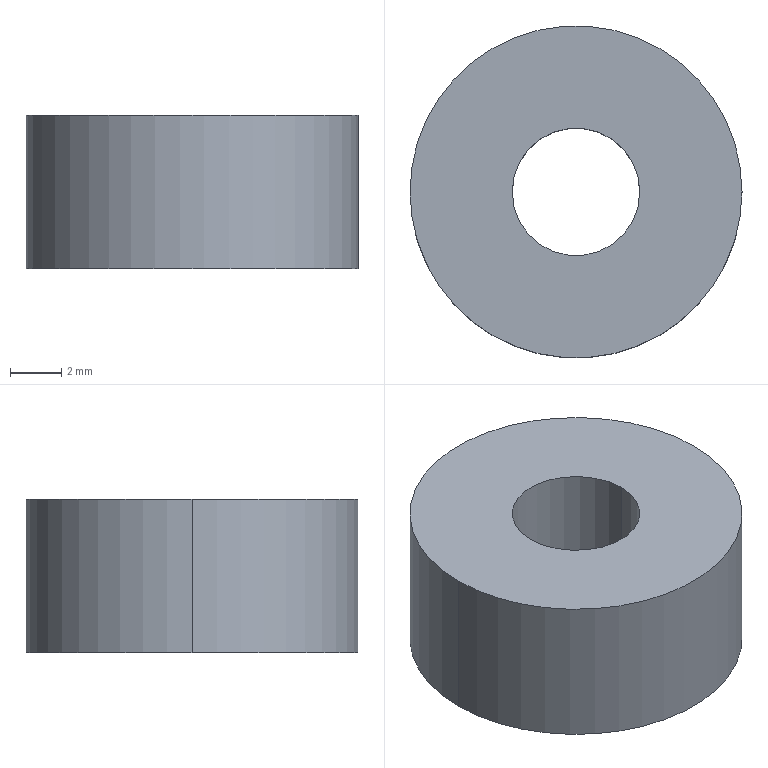Part | SolidWorks | features Extrusion 1 | 1 solid | 6 faces | box 13 x 13 x 6 mm | volume 678.584 mm3 | cylinder 4 | plane 2 | commonest cylinder face diameters 5 x2 13 x2
STEP:
#1=CARTESIAN_POINT('',(-2.5,0.,6.));
#2=VERTEX_POINT('',#1);
#3=CARTESIAN_POINT('',(2.5,0.,6.));
#4=VERTEX_POINT('',#3);
#5=CARTESIAN_POINT('',(0.,0.,6.));
#6=DIRECTION('',(0.,0.,1.));
#7=DIRECTION('',(1.,0.,0.));
#8=AXIS2_PLACEMENT_3D('',#5,#6,#7);
#9=CIRCLE('',#8,2.5);
#10=EDGE_CURVE('',#2,#4,#9,.T.);
#11=ORIENTED_EDGE('',*,*,#10,.T.);
#12=CARTESIAN_POINT('',(2.5,0.,0.));
#13=VERTEX_POINT('',#12);
#14=CARTESIAN_POINT('',(2.5,0.,6.));
#15=DIRECTION('',(0.,0.,-1.));
#16=VECTOR('',#15,1000.);
#17=LINE('',#14,#16);
#18=EDGE_CURVE('',#4,#13,#17,.T.);
#19=ORIENTED_EDGE('',*,*,#18,.T.);
#20=CARTESIAN_POINT('',(-2.5,0.,0.));
#21=VERTEX_POINT('',#20);
#22=CARTESIAN_POINT('',(0.,0.,0.));
#23=DIRECTION('',(0.,0.,1.));
#24=DIRECTION('',(1.,0.,0.));
#25=AXIS2_PLACEMENT_3D('',#22,#23,#24);
#26=CIRCLE('',#25,2.5);
#27=EDGE_CURVE('',#21,#13,#26,.T.);
#28=ORIENTED_EDGE('',*,*,#27,.F.);
#29=CARTESIAN_POINT('',(-2.5,0.,6.));
#30=DIRECTION('',(0.,0.,-1.));
#31=VECTOR('',#30,1000.);
#32=LINE('',#29,#31);
#33=EDGE_CURVE('',#2,#21,#32,.T.);
#34=ORIENTED_EDGE('',*,*,#33,.F.);
#35=EDGE_LOOP('',(#11,#19,#28,#34));
#36=FACE_OUTER_BOUND('',#35,.T.);
#37=CARTESIAN_POINT('',(0.,0.,6.));
#38=DIRECTION('',(0.,0.,-1.));
#39=DIRECTION('',(-1.,0.,0.));
#40=AXIS2_PLACEMENT_3D('',#37,#38,#39);
#41=CYLINDRICAL_SURFACE('',#40,2.5);
#42=ADVANCED_FACE('',(#36),#41,.F.);
#43=CARTESIAN_POINT('',(6.5,0.,6.));
#44=VERTEX_POINT('',#43);
#45=CARTESIAN_POINT('',(-6.5,0.,6.));
#46=VERTEX_POINT('',#45);
#47=CARTESIAN_POINT('',(0.,0.,6.));
#48=DIRECTION('',(0.,0.,1.));
#49=DIRECTION('',(1.,0.,0.));
#50=AXIS2_PLACEMENT_3D('',#47,#48,#49);
#51=CIRCLE('',#50,6.5);
#52=EDGE_CURVE('',#44,#46,#51,.T.);
#53=ORIENTED_EDGE('',*,*,#52,.F.);
#54=CARTESIAN_POINT('',(6.5,0.,0.));
#55=VERTEX_POINT('',#54);
#56=CARTESIAN_POINT('',(6.5,0.,6.));
#57=DIRECTION('',(0.,0.,-1.));
#58=VECTOR('',#57,1000.);
#59=LINE('',#56,#58);
#60=EDGE_CURVE('',#44,#55,#59,.T.);
#61=ORIENTED_EDGE('',*,*,#60,.T.);
#62=CARTESIAN_POINT('',(-6.5,0.,0.));
#63=VERTEX_POINT('',#62);
#64=CARTESIAN_POINT('',(0.,0.,0.));
#65=DIRECTION('',(0.,0.,1.));
#66=DIRECTION('',(1.,0.,0.));
#67=AXIS2_PLACEMENT_3D('',#64,#65,#66);
#68=CIRCLE('',#67,6.5);
#69=EDGE_CURVE('',#55,#63,#68,.T.);
#70=ORIENTED_EDGE('',*,*,#69,.T.);
#71=CARTESIAN_POINT('',(-6.5,0.,6.));
#72=DIRECTION('',(0.,0.,-1.));
#73=VECTOR('',#72,1000.);
#74=LINE('',#71,#73);
#75=EDGE_CURVE('',#46,#63,#74,.T.);
#76=ORIENTED_EDGE('',*,*,#75,.F.);
#77=EDGE_LOOP('',(#53,#61,#70,#76));
#78=FACE_OUTER_BOUND('',#77,.T.);
#79=CARTESIAN_POINT('',(0.,0.,6.));
#80=DIRECTION('',(0.,0.,-1.));
#81=DIRECTION('',(-1.,0.,0.));
#82=AXIS2_PLACEMENT_3D('',#79,#80,#81);
#83=CYLINDRICAL_SURFACE('',#82,6.5);
#84=ADVANCED_FACE('',(#78),#83,.T.);
#85=CARTESIAN_POINT('',(0.,0.,6.));
#86=DIRECTION('',(0.,0.,1.));
#87=DIRECTION('',(1.,0.,0.));
#88=AXIS2_PLACEMENT_3D('',#85,#86,#87);
#89=CIRCLE('',#88,6.5);
#90=EDGE_CURVE('',#46,#44,#89,.T.);
#91=ORIENTED_EDGE('',*,*,#90,.T.);
#92=ORIENTED_EDGE('',*,*,#52,.T.);
#93=EDGE_LOOP('',(#91,#92));
#94=FACE_OUTER_BOUND('',#93,.T.);
#95=ORIENTED_EDGE('',*,*,#10,.F.);
#96=CARTESIAN_POINT('',(0.,0.,6.));
#97=DIRECTION('',(0.,0.,1.));
#98=DIRECTION('',(1.,0.,0.));
#99=AXIS2_PLACEMENT_3D('',#96,#97,#98);
#100=CIRCLE('',#99,2.5);
#101=EDGE_CURVE('',#4,#2,#100,.T.);
#102=ORIENTED_EDGE('',*,*,#101,.F.);
#103=EDGE_LOOP('',(#95,#102));
#104=FACE_BOUND('',#103,.T.);
#105=CARTESIAN_POINT('',(0.,0.,6.));
#106=DIRECTION('',(0.,0.,1.));
#107=DIRECTION('',(1.,0.,0.));
#108=AXIS2_PLACEMENT_3D('',#105,#106,#107);
#109=PLANE('',#108);
#110=ADVANCED_FACE('',(#94,#104),#109,.T.);
#111=CARTESIAN_POINT('',(0.,0.,0.));
#112=DIRECTION('',(0.,0.,1.));
#113=DIRECTION('',(1.,0.,0.));
#114=AXIS2_PLACEMENT_3D('',#111,#112,#113);
#115=CIRCLE('',#114,6.5);
#116=EDGE_CURVE('',#63,#55,#115,.T.);
#117=ORIENTED_EDGE('',*,*,#116,.F.);
#118=ORIENTED_EDGE('',*,*,#69,.F.);
#119=EDGE_LOOP('',(#117,#118));
#120=FACE_OUTER_BOUND('',#119,.T.);
#121=ORIENTED_EDGE('',*,*,#27,.T.);
#122=CARTESIAN_POINT('',(0.,0.,0.));
#123=DIRECTION('',(0.,0.,1.));
#124=DIRECTION('',(1.,0.,0.));
#125=AXIS2_PLACEMENT_3D('',#122,#123,#124);
#126=CIRCLE('',#125,2.5);
#127=EDGE_CURVE('',#13,#21,#126,.T.);
#128=ORIENTED_EDGE('',*,*,#127,.T.);
#129=EDGE_LOOP('',(#121,#128));
#130=FACE_BOUND('',#129,.T.);
#131=CARTESIAN_POINT('',(0.,0.,0.));
#132=DIRECTION('',(0.,0.,1.));
#133=DIRECTION('',(1.,0.,0.));
#134=AXIS2_PLACEMENT_3D('',#131,#132,#133);
#135=PLANE('',#134);
#136=ADVANCED_FACE('',(#120,#130),#135,.F.);
#137=ORIENTED_EDGE('',*,*,#60,.F.);
#138=ORIENTED_EDGE('',*,*,#90,.F.);
#139=ORIENTED_EDGE('',*,*,#75,.T.);
#140=ORIENTED_EDGE('',*,*,#116,.T.);
#141=EDGE_LOOP('',(#137,#138,#139,#140));
#142=FACE_OUTER_BOUND('',#141,.T.);
#143=CARTESIAN_POINT('',(0.,0.,6.));
#144=DIRECTION('',(0.,0.,-1.));
#145=DIRECTION('',(-1.,0.,0.));
#146=AXIS2_PLACEMENT_3D('',#143,#144,#145);
#147=CYLINDRICAL_SURFACE('',#146,6.5);
#148=ADVANCED_FACE('',(#142),#147,.T.);
#149=ORIENTED_EDGE('',*,*,#18,.F.);
#150=ORIENTED_EDGE('',*,*,#101,.T.);
#151=ORIENTED_EDGE('',*,*,#33,.T.);
#152=ORIENTED_EDGE('',*,*,#127,.F.);
#153=EDGE_LOOP('',(#149,#150,#151,#152));
#154=FACE_OUTER_BOUND('',#153,.T.);
#155=CARTESIAN_POINT('',(0.,0.,6.));
#156=DIRECTION('',(0.,0.,-1.));
#157=DIRECTION('',(-1.,0.,0.));
#158=AXIS2_PLACEMENT_3D('',#155,#156,#157);
#159=CYLINDRICAL_SURFACE('',#158,2.5);
#160=ADVANCED_FACE('',(#154),#159,.F.);
#161=CLOSED_SHELL('',(#42,#84,#110,#136,#148,#160));
#162=MANIFOLD_SOLID_BREP('',#161);
#163=CARTESIAN_POINT('',(0.,0.,0.));
#164=DIRECTION('',(0.,0.,1.));
#165=DIRECTION('',(1.,0.,0.));
#166=AXIS2_PLACEMENT_3D('',#163,#164,#165);
#167=(LENGTH_UNIT()NAMED_UNIT(*)SI_UNIT(.MILLI.,.METRE.));
#168=UNCERTAINTY_MEASURE_WITH_UNIT(LENGTH_MEASURE(0.00001),#167,'','');
#169=(NAMED_UNIT(*)PLANE_ANGLE_UNIT()SI_UNIT($,.RADIAN.));
#170=(NAMED_UNIT(*)SI_UNIT($,.STERADIAN.)SOLID_ANGLE_UNIT());
#171=(GEOMETRIC_REPRESENTATION_CONTEXT(3)GLOBAL_UNCERTAINTY_ASSIGNED_CONTEXT((#168))GLOBAL_UNIT_ASSIGNED_CONTEXT((#167,#169,#170))REPRESENTATION_CONTEXT('',''));
#172=ADVANCED_BREP_SHAPE_REPRESENTATION('',(#162,#166),#171);